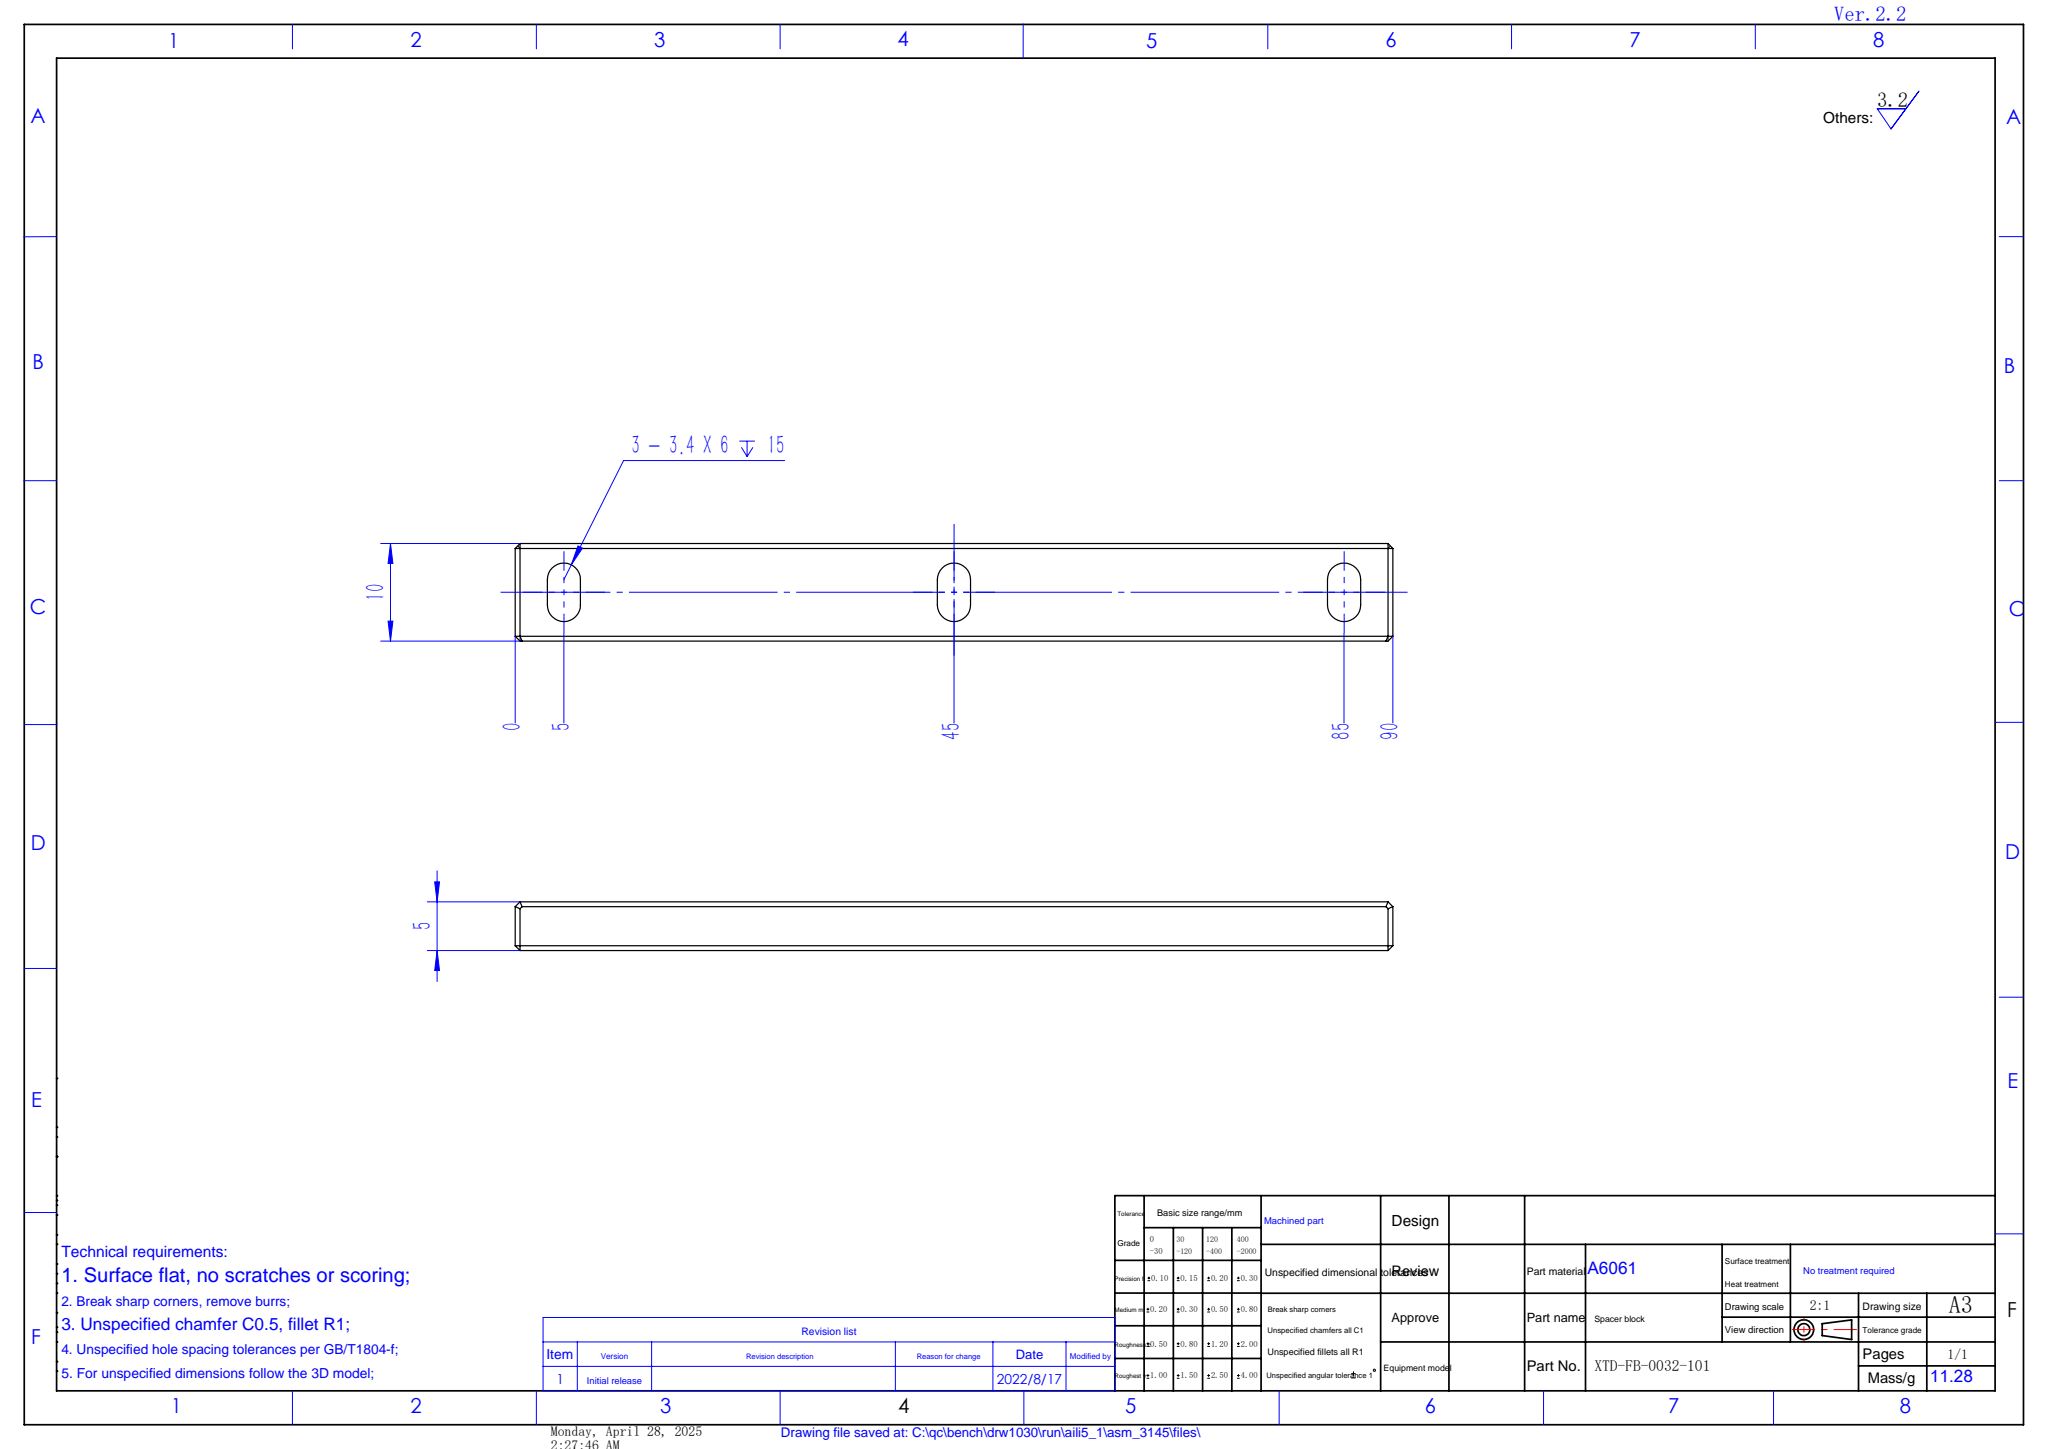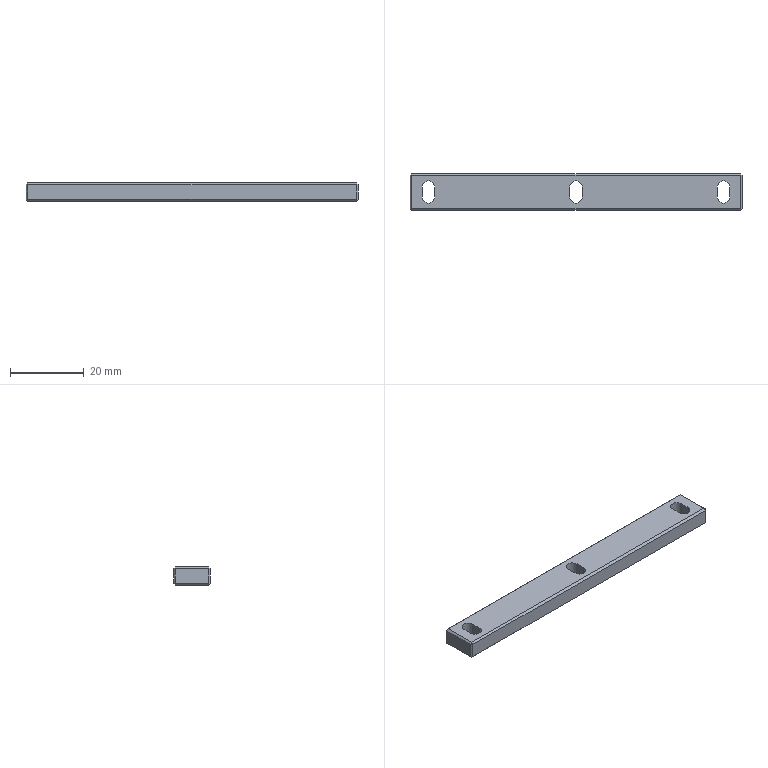Part | SolidWorks | features Chamfer 2, Extrusion 1, HoleWzd 1 | 1 solid | 36 faces | box 90 x 10 x 5 mm | volume 4179 mm3 | plane 30 | cylinder 6 | commonest cylinder face diameters 3.4 x6
STEP:
#1=CARTESIAN_POINT('',(44.5,-4.5,5.));
#2=VERTEX_POINT('',#1);
#3=CARTESIAN_POINT('',(44.5,4.5,5.));
#4=VERTEX_POINT('',#3);
#5=CARTESIAN_POINT('',(44.5,0.,5.));
#6=DIRECTION('',(0.,1.,0.));
#7=VECTOR('',#6,1000.);
#8=LINE('',#5,#7);
#9=EDGE_CURVE('',#2,#4,#8,.T.);
#10=ORIENTED_EDGE('',*,*,#9,.T.);
#11=CARTESIAN_POINT('',(-44.5,4.5,5.));
#12=VERTEX_POINT('',#11);
#13=CARTESIAN_POINT('',(0.,4.5,5.));
#14=DIRECTION('',(-1.,0.,0.));
#15=VECTOR('',#14,1000.);
#16=LINE('',#13,#15);
#17=EDGE_CURVE('',#4,#12,#16,.T.);
#18=ORIENTED_EDGE('',*,*,#17,.T.);
#19=CARTESIAN_POINT('',(-44.5,-4.5,5.));
#20=VERTEX_POINT('',#19);
#21=CARTESIAN_POINT('',(-44.5,0.,5.));
#22=DIRECTION('',(0.,-1.,0.));
#23=VECTOR('',#22,1000.);
#24=LINE('',#21,#23);
#25=EDGE_CURVE('',#12,#20,#24,.T.);
#26=ORIENTED_EDGE('',*,*,#25,.T.);
#27=CARTESIAN_POINT('',(0.,-4.5,5.));
#28=DIRECTION('',(1.,0.,0.));
#29=VECTOR('',#28,1000.);
#30=LINE('',#27,#29);
#31=EDGE_CURVE('',#20,#2,#30,.T.);
#32=ORIENTED_EDGE('',*,*,#31,.T.);
#33=EDGE_LOOP('',(#10,#18,#26,#32));
#34=FACE_OUTER_BOUND('',#33,.T.);
#35=CARTESIAN_POINT('',(1.7,-1.3,5.));
#36=VERTEX_POINT('',#35);
#37=CARTESIAN_POINT('',(-1.7,-1.3,5.));
#38=VERTEX_POINT('',#37);
#39=CARTESIAN_POINT('',(0.,-1.3,5.));
#40=DIRECTION('',(0.,0.,-1.));
#41=DIRECTION('',(-1.,0.,0.));
#42=AXIS2_PLACEMENT_3D('',#39,#40,#41);
#43=CIRCLE('',#42,1.7);
#44=EDGE_CURVE('',#36,#38,#43,.T.);
#45=ORIENTED_EDGE('',*,*,#44,.T.);
#46=CARTESIAN_POINT('',(-1.7,1.3,5.));
#47=VERTEX_POINT('',#46);
#48=CARTESIAN_POINT('',(-1.7,0.,5.));
#49=DIRECTION('',(0.,1.,0.));
#50=VECTOR('',#49,1000.);
#51=LINE('',#48,#50);
#52=EDGE_CURVE('',#38,#47,#51,.T.);
#53=ORIENTED_EDGE('',*,*,#52,.T.);
#54=CARTESIAN_POINT('',(1.7,1.3,5.));
#55=VERTEX_POINT('',#54);
#56=CARTESIAN_POINT('',(0.,1.3,5.));
#57=DIRECTION('',(0.,0.,-1.));
#58=DIRECTION('',(-1.,0.,0.));
#59=AXIS2_PLACEMENT_3D('',#56,#57,#58);
#60=CIRCLE('',#59,1.7);
#61=EDGE_CURVE('',#47,#55,#60,.T.);
#62=ORIENTED_EDGE('',*,*,#61,.T.);
#63=CARTESIAN_POINT('',(1.7,0.,5.));
#64=DIRECTION('',(0.,1.,0.));
#65=VECTOR('',#64,1000.);
#66=LINE('',#63,#65);
#67=EDGE_CURVE('',#36,#55,#66,.T.);
#68=ORIENTED_EDGE('',*,*,#67,.F.);
#69=EDGE_LOOP('',(#45,#53,#62,#68));
#70=FACE_BOUND('',#69,.T.);
#71=CARTESIAN_POINT('',(-41.7,-1.3,5.));
#72=VERTEX_POINT('',#71);
#73=CARTESIAN_POINT('',(-41.7,1.3,5.));
#74=VERTEX_POINT('',#73);
#75=CARTESIAN_POINT('',(-41.7,0.,5.));
#76=DIRECTION('',(0.,1.,0.));
#77=VECTOR('',#76,1000.);
#78=LINE('',#75,#77);
#79=EDGE_CURVE('',#72,#74,#78,.T.);
#80=ORIENTED_EDGE('',*,*,#79,.T.);
#81=CARTESIAN_POINT('',(-38.3,1.3,5.));
#82=VERTEX_POINT('',#81);
#83=CARTESIAN_POINT('',(-40.,1.3,5.));
#84=DIRECTION('',(0.,0.,-1.));
#85=DIRECTION('',(-1.,0.,0.));
#86=AXIS2_PLACEMENT_3D('',#83,#84,#85);
#87=CIRCLE('',#86,1.7);
#88=EDGE_CURVE('',#74,#82,#87,.T.);
#89=ORIENTED_EDGE('',*,*,#88,.T.);
#90=CARTESIAN_POINT('',(-38.3,-1.3,5.));
#91=VERTEX_POINT('',#90);
#92=CARTESIAN_POINT('',(-38.3,0.,5.));
#93=DIRECTION('',(0.,1.,0.));
#94=VECTOR('',#93,1000.);
#95=LINE('',#92,#94);
#96=EDGE_CURVE('',#91,#82,#95,.T.);
#97=ORIENTED_EDGE('',*,*,#96,.F.);
#98=CARTESIAN_POINT('',(-40.,-1.3,5.));
#99=DIRECTION('',(0.,0.,-1.));
#100=DIRECTION('',(-1.,0.,0.));
#101=AXIS2_PLACEMENT_3D('',#98,#99,#100);
#102=CIRCLE('',#101,1.7);
#103=EDGE_CURVE('',#91,#72,#102,.T.);
#104=ORIENTED_EDGE('',*,*,#103,.T.);
#105=EDGE_LOOP('',(#80,#89,#97,#104));
#106=FACE_BOUND('',#105,.T.);
#107=CARTESIAN_POINT('',(41.7,-1.3,5.));
#108=VERTEX_POINT('',#107);
#109=CARTESIAN_POINT('',(41.7,1.3,5.));
#110=VERTEX_POINT('',#109);
#111=CARTESIAN_POINT('',(41.7,0.,5.));
#112=DIRECTION('',(0.,1.,0.));
#113=VECTOR('',#112,1000.);
#114=LINE('',#111,#113);
#115=EDGE_CURVE('',#108,#110,#114,.T.);
#116=ORIENTED_EDGE('',*,*,#115,.F.);
#117=CARTESIAN_POINT('',(38.3,-1.3,5.));
#118=VERTEX_POINT('',#117);
#119=CARTESIAN_POINT('',(40.,-1.3,5.));
#120=DIRECTION('',(0.,0.,-1.));
#121=DIRECTION('',(-1.,0.,0.));
#122=AXIS2_PLACEMENT_3D('',#119,#120,#121);
#123=CIRCLE('',#122,1.7);
#124=EDGE_CURVE('',#108,#118,#123,.T.);
#125=ORIENTED_EDGE('',*,*,#124,.T.);
#126=CARTESIAN_POINT('',(38.3,1.3,5.));
#127=VERTEX_POINT('',#126);
#128=CARTESIAN_POINT('',(38.3,0.,5.));
#129=DIRECTION('',(0.,1.,0.));
#130=VECTOR('',#129,1000.);
#131=LINE('',#128,#130);
#132=EDGE_CURVE('',#118,#127,#131,.T.);
#133=ORIENTED_EDGE('',*,*,#132,.T.);
#134=CARTESIAN_POINT('',(40.,1.3,5.));
#135=DIRECTION('',(0.,0.,-1.));
#136=DIRECTION('',(-1.,0.,0.));
#137=AXIS2_PLACEMENT_3D('',#134,#135,#136);
#138=CIRCLE('',#137,1.7);
#139=EDGE_CURVE('',#127,#110,#138,.T.);
#140=ORIENTED_EDGE('',*,*,#139,.T.);
#141=EDGE_LOOP('',(#116,#125,#133,#140));
#142=FACE_BOUND('',#141,.T.);
#143=CARTESIAN_POINT('',(0.,0.,5.));
#144=DIRECTION('',(0.,0.,-1.));
#145=DIRECTION('',(-1.,0.,0.));
#146=AXIS2_PLACEMENT_3D('',#143,#144,#145);
#147=PLANE('',#146);
#148=ADVANCED_FACE('',(#34,#70,#106,#142),#147,.F.);
#149=CARTESIAN_POINT('',(45.,-4.5,4.5));
#150=VERTEX_POINT('',#149);
#151=CARTESIAN_POINT('',(45.,-4.5,0.5));
#152=VERTEX_POINT('',#151);
#153=CARTESIAN_POINT('',(45.,-4.5,5.));
#154=DIRECTION('',(0.,0.,-1.));
#155=VECTOR('',#154,1000.);
#156=LINE('',#153,#155);
#157=EDGE_CURVE('',#150,#152,#156,.T.);
#158=ORIENTED_EDGE('',*,*,#157,.T.);
#159=CARTESIAN_POINT('',(45.,4.5,0.5));
#160=VERTEX_POINT('',#159);
#161=CARTESIAN_POINT('',(45.,5.,0.5));
#162=DIRECTION('',(0.,1.,0.));
#163=VECTOR('',#162,1000.);
#164=LINE('',#161,#163);
#165=EDGE_CURVE('',#152,#160,#164,.T.);
#166=ORIENTED_EDGE('',*,*,#165,.T.);
#167=CARTESIAN_POINT('',(45.,4.5,4.5));
#168=VERTEX_POINT('',#167);
#169=CARTESIAN_POINT('',(45.,4.5,5.));
#170=DIRECTION('',(0.,0.,1.));
#171=VECTOR('',#170,1000.);
#172=LINE('',#169,#171);
#173=EDGE_CURVE('',#160,#168,#172,.T.);
#174=ORIENTED_EDGE('',*,*,#173,.T.);
#175=CARTESIAN_POINT('',(45.,-5.,4.5));
#176=DIRECTION('',(0.,-1.,0.));
#177=VECTOR('',#176,1000.);
#178=LINE('',#175,#177);
#179=EDGE_CURVE('',#168,#150,#178,.T.);
#180=ORIENTED_EDGE('',*,*,#179,.T.);
#181=EDGE_LOOP('',(#158,#166,#174,#180));
#182=FACE_OUTER_BOUND('',#181,.T.);
#183=CARTESIAN_POINT('',(45.,-5.,5.));
#184=DIRECTION('',(-1.,0.,0.));
#185=DIRECTION('',(0.,0.,1.));
#186=AXIS2_PLACEMENT_3D('',#183,#184,#185);
#187=PLANE('',#186);
#188=ADVANCED_FACE('',(#182),#187,.F.);
#189=CARTESIAN_POINT('',(44.5,5.,4.293));
#190=VERTEX_POINT('',#189);
#191=CARTESIAN_POINT('',(44.5,5.,0.5));
#192=VERTEX_POINT('',#191);
#193=CARTESIAN_POINT('',(44.5,5.,5.));
#194=DIRECTION('',(0.,0.,-1.));
#195=VECTOR('',#194,1000.);
#196=LINE('',#193,#195);
#197=EDGE_CURVE('',#190,#192,#196,.T.);
#198=ORIENTED_EDGE('',*,*,#197,.T.);
#199=CARTESIAN_POINT('',(-44.5,5.,0.5));
#200=VERTEX_POINT('',#199);
#201=CARTESIAN_POINT('',(-45.,5.,0.5));
#202=DIRECTION('',(-1.,0.,0.));
#203=VECTOR('',#202,1000.);
#204=LINE('',#201,#203);
#205=EDGE_CURVE('',#192,#200,#204,.T.);
#206=ORIENTED_EDGE('',*,*,#205,.T.);
#207=CARTESIAN_POINT('',(-44.5,5.,4.293));
#208=VERTEX_POINT('',#207);
#209=CARTESIAN_POINT('',(-44.5,5.,5.));
#210=DIRECTION('',(0.,0.,1.));
#211=VECTOR('',#210,1000.);
#212=LINE('',#209,#211);
#213=EDGE_CURVE('',#200,#208,#212,.T.);
#214=ORIENTED_EDGE('',*,*,#213,.T.);
#215=CARTESIAN_POINT('',(-44.293,5.,4.5));
#216=VERTEX_POINT('',#215);
#217=CARTESIAN_POINT('',(-44.146,5.,4.646));
#218=DIRECTION('',(0.7071,0.,0.7071));
#219=VECTOR('',#218,1000.);
#220=LINE('',#217,#219);
#221=EDGE_CURVE('',#208,#216,#220,.T.);
#222=ORIENTED_EDGE('',*,*,#221,.T.);
#223=CARTESIAN_POINT('',(44.293,5.,4.5));
#224=VERTEX_POINT('',#223);
#225=CARTESIAN_POINT('',(-45.,5.,4.5));
#226=DIRECTION('',(1.,0.,0.));
#227=VECTOR('',#226,1000.);
#228=LINE('',#225,#227);
#229=EDGE_CURVE('',#216,#224,#228,.T.);
#230=ORIENTED_EDGE('',*,*,#229,.T.);
#231=CARTESIAN_POINT('',(44.646,5.,4.146));
#232=DIRECTION('',(0.7071,0.,-0.7071));
#233=VECTOR('',#232,1000.);
#234=LINE('',#231,#233);
#235=EDGE_CURVE('',#224,#190,#234,.T.);
#236=ORIENTED_EDGE('',*,*,#235,.T.);
#237=EDGE_LOOP('',(#198,#206,#214,#222,#230,#236));
#238=FACE_OUTER_BOUND('',#237,.T.);
#239=CARTESIAN_POINT('',(-45.,5.,5.));
#240=DIRECTION('',(0.,-1.,0.));
#241=DIRECTION('',(0.,0.,-1.));
#242=AXIS2_PLACEMENT_3D('',#239,#240,#241);
#243=PLANE('',#242);
#244=ADVANCED_FACE('',(#238),#243,.F.);
#245=CARTESIAN_POINT('',(-45.,-4.5,4.5));
#246=VERTEX_POINT('',#245);
#247=CARTESIAN_POINT('',(-45.,4.5,4.5));
#248=VERTEX_POINT('',#247);
#249=CARTESIAN_POINT('',(-45.,-5.,4.5));
#250=DIRECTION('',(0.,1.,0.));
#251=VECTOR('',#250,1000.);
#252=LINE('',#249,#251);
#253=EDGE_CURVE('',#246,#248,#252,.T.);
#254=ORIENTED_EDGE('',*,*,#253,.T.);
#255=CARTESIAN_POINT('',(-45.,4.5,0.5));
#256=VERTEX_POINT('',#255);
#257=CARTESIAN_POINT('',(-45.,4.5,5.));
#258=DIRECTION('',(0.,0.,-1.));
#259=VECTOR('',#258,1000.);
#260=LINE('',#257,#259);
#261=EDGE_CURVE('',#248,#256,#260,.T.);
#262=ORIENTED_EDGE('',*,*,#261,.T.);
#263=CARTESIAN_POINT('',(-45.,-4.5,0.5));
#264=VERTEX_POINT('',#263);
#265=CARTESIAN_POINT('',(-45.,-4.5,0.5));
#266=DIRECTION('',(0.,-1.,0.));
#267=VECTOR('',#266,1000.);
#268=LINE('',#265,#267);
#269=EDGE_CURVE('',#256,#264,#268,.T.);
#270=ORIENTED_EDGE('',*,*,#269,.T.);
#271=CARTESIAN_POINT('',(-45.,-4.5,5.));
#272=DIRECTION('',(0.,0.,1.));
#273=VECTOR('',#272,1000.);
#274=LINE('',#271,#273);
#275=EDGE_CURVE('',#264,#246,#274,.T.);
#276=ORIENTED_EDGE('',*,*,#275,.T.);
#277=EDGE_LOOP('',(#254,#262,#270,#276));
#278=FACE_OUTER_BOUND('',#277,.T.);
#279=CARTESIAN_POINT('',(-45.,-5.,5.));
#280=DIRECTION('',(1.,0.,0.));
#281=DIRECTION('',(0.,0.,-1.));
#282=AXIS2_PLACEMENT_3D('',#279,#280,#281);
#283=PLANE('',#282);
#284=ADVANCED_FACE('',(#278),#283,.F.);
#285=CARTESIAN_POINT('',(44.5,-5.,4.5));
#286=VERTEX_POINT('',#285);
#287=CARTESIAN_POINT('',(-44.5,-5.,4.5));
#288=VERTEX_POINT('',#287);
#289=CARTESIAN_POINT('',(-45.,-5.,4.5));
#290=DIRECTION('',(-1.,0.,0.));
#291=VECTOR('',#290,1000.);
#292=LINE('',#289,#291);
#293=EDGE_CURVE('',#286,#288,#292,.T.);
#294=ORIENTED_EDGE('',*,*,#293,.T.);
#295=CARTESIAN_POINT('',(-44.5,-5.,0.5));
#296=VERTEX_POINT('',#295);
#297=CARTESIAN_POINT('',(-44.5,-5.,5.));
#298=DIRECTION('',(0.,0.,-1.));
#299=VECTOR('',#298,1000.);
#300=LINE('',#297,#299);
#301=EDGE_CURVE('',#288,#296,#300,.T.);
#302=ORIENTED_EDGE('',*,*,#301,.T.);
#303=CARTESIAN_POINT('',(44.5,-5.,0.5));
#304=VERTEX_POINT('',#303);
#305=CARTESIAN_POINT('',(45.,-5.,0.5));
#306=DIRECTION('',(1.,0.,0.));
#307=VECTOR('',#306,1000.);
#308=LINE('',#305,#307);
#309=EDGE_CURVE('',#296,#304,#308,.T.);
#310=ORIENTED_EDGE('',*,*,#309,.T.);
#311=CARTESIAN_POINT('',(44.5,-5.,5.));
#312=DIRECTION('',(0.,0.,1.));
#313=VECTOR('',#312,1000.);
#314=LINE('',#311,#313);
#315=EDGE_CURVE('',#304,#286,#314,.T.);
#316=ORIENTED_EDGE('',*,*,#315,.T.);
#317=EDGE_LOOP('',(#294,#302,#310,#316));
#318=FACE_OUTER_BOUND('',#317,.T.);
#319=CARTESIAN_POINT('',(-45.,-5.,5.));
#320=DIRECTION('',(0.,1.,0.));
#321=DIRECTION('',(0.,0.,1.));
#322=AXIS2_PLACEMENT_3D('',#319,#320,#321);
#323=PLANE('',#322);
#324=ADVANCED_FACE('',(#318),#323,.F.);
#325=CARTESIAN_POINT('',(38.3,-1.3,0.));
#326=VERTEX_POINT('',#325);
#327=CARTESIAN_POINT('',(38.3,1.3,0.));
#328=VERTEX_POINT('',#327);
#329=CARTESIAN_POINT('',(38.3,-1.3,0.));
#330=DIRECTION('',(0.,1.,0.));
#331=VECTOR('',#330,1000.);
#332=LINE('',#329,#331);
#333=EDGE_CURVE('',#326,#328,#332,.T.);
#334=ORIENTED_EDGE('',*,*,#333,.F.);
#335=CARTESIAN_POINT('',(41.7,-1.3,0.));
#336=VERTEX_POINT('',#335);
#337=CARTESIAN_POINT('',(40.,-1.3,0.));
#338=DIRECTION('',(0.,0.,-1.));
#339=DIRECTION('',(-1.,0.,0.));
#340=AXIS2_PLACEMENT_3D('',#337,#338,#339);
#341=CIRCLE('',#340,1.7);
#342=EDGE_CURVE('',#336,#326,#341,.T.);
#343=ORIENTED_EDGE('',*,*,#342,.F.);
#344=CARTESIAN_POINT('',(41.7,1.3,0.));
#345=VERTEX_POINT('',#344);
#346=CARTESIAN_POINT('',(41.7,-1.3,0.));
#347=DIRECTION('',(0.,1.,0.));
#348=VECTOR('',#347,1000.);
#349=LINE('',#346,#348);
#350=EDGE_CURVE('',#336,#345,#349,.T.);
#351=ORIENTED_EDGE('',*,*,#350,.T.);
#352=CARTESIAN_POINT('',(40.,1.3,0.));
#353=DIRECTION('',(0.,0.,-1.));
#354=DIRECTION('',(-1.,0.,0.));
#355=AXIS2_PLACEMENT_3D('',#352,#353,#354);
#356=CIRCLE('',#355,1.7);
#357=EDGE_CURVE('',#328,#345,#356,.T.);
#358=ORIENTED_EDGE('',*,*,#357,.F.);
#359=EDGE_LOOP('',(#334,#343,#351,#358));
#360=FACE_BOUND('',#359,.T.);
#361=CARTESIAN_POINT('',(-41.7,1.3,0.));
#362=VERTEX_POINT('',#361);
#363=CARTESIAN_POINT('',(-38.3,1.3,0.));
#364=VERTEX_POINT('',#363);
#365=CARTESIAN_POINT('',(-40.,1.3,0.));
#366=DIRECTION('',(0.,0.,-1.));
#367=DIRECTION('',(-1.,0.,0.));
#368=AXIS2_PLACEMENT_3D('',#365,#366,#367);
#369=CIRCLE('',#368,1.7);
#370=EDGE_CURVE('',#362,#364,#369,.T.);
#371=ORIENTED_EDGE('',*,*,#370,.F.);
#372=CARTESIAN_POINT('',(-41.7,-1.3,0.));
#373=VERTEX_POINT('',#372);
#374=CARTESIAN_POINT('',(-41.7,-1.3,0.));
#375=DIRECTION('',(0.,1.,0.));
#376=VECTOR('',#375,1000.);
#377=LINE('',#374,#376);
#378=EDGE_CURVE('',#373,#362,#377,.T.);
#379=ORIENTED_EDGE('',*,*,#378,.F.);
#380=CARTESIAN_POINT('',(-38.3,-1.3,0.));
#381=VERTEX_POINT('',#380);
#382=CARTESIAN_POINT('',(-40.,-1.3,0.));
#383=DIRECTION('',(0.,0.,-1.));
#384=DIRECTION('',(-1.,0.,0.));
#385=AXIS2_PLACEMENT_3D('',#382,#383,#384);
#386=CIRCLE('',#385,1.7);
#387=EDGE_CURVE('',#381,#373,#386,.T.);
#388=ORIENTED_EDGE('',*,*,#387,.F.);
#389=CARTESIAN_POINT('',(-38.3,-1.3,0.));
#390=DIRECTION('',(0.,1.,0.));
#391=VECTOR('',#390,1000.);
#392=LINE('',#389,#391);
#393=EDGE_CURVE('',#381,#364,#392,.T.);
#394=ORIENTED_EDGE('',*,*,#393,.T.);
#395=EDGE_LOOP('',(#371,#379,#388,#394));
#396=FACE_BOUND('',#395,.T.);
#397=CARTESIAN_POINT('',(1.7,-1.3,0.));
#398=VERTEX_POINT('',#397);
#399=CARTESIAN_POINT('',(-1.7,-1.3,0.));
#400=VERTEX_POINT('',#399);
#401=CARTESIAN_POINT('',(0.,-1.3,0.));
#402=DIRECTION('',(0.,0.,-1.));
#403=DIRECTION('',(-1.,0.,0.));
#404=AXIS2_PLACEMENT_3D('',#401,#402,#403);
#405=CIRCLE('',#404,1.7);
#406=EDGE_CURVE('',#398,#400,#405,.T.);
#407=ORIENTED_EDGE('',*,*,#406,.F.);
#408=CARTESIAN_POINT('',(1.7,1.3,0.));
#409=VERTEX_POINT('',#408);
#410=CARTESIAN_POINT('',(1.7,-1.3,0.));
#411=DIRECTION('',(0.,1.,0.));
#412=VECTOR('',#411,1000.);
#413=LINE('',#410,#412);
#414=EDGE_CURVE('',#398,#409,#413,.T.);
#415=ORIENTED_EDGE('',*,*,#414,.T.);
#416=CARTESIAN_POINT('',(-1.7,1.3,0.));
#417=VERTEX_POINT('',#416);
#418=CARTESIAN_POINT('',(0.,1.3,0.));
#419=DIRECTION('',(0.,0.,-1.));
#420=DIRECTION('',(-1.,0.,0.));
#421=AXIS2_PLACEMENT_3D('',#418,#419,#420);
#422=CIRCLE('',#421,1.7);
#423=EDGE_CURVE('',#417,#409,#422,.T.);
#424=ORIENTED_EDGE('',*,*,#423,.F.);
#425=CARTESIAN_POINT('',(-1.7,-1.3,0.));
#426=DIRECTION('',(0.,1.,0.));
#427=VECTOR('',#426,1000.);
#428=LINE('',#425,#427);
#429=EDGE_CURVE('',#400,#417,#428,.T.);
#430=ORIENTED_EDGE('',*,*,#429,.F.);
#431=EDGE_LOOP('',(#407,#415,#424,#430));
#432=FACE_BOUND('',#431,.T.);
#433=CARTESIAN_POINT('',(-44.5,4.5,0.));
#434=VERTEX_POINT('',#433);
#435=CARTESIAN_POINT('',(44.5,4.5,0.));
#436=VERTEX_POINT('',#435);
#437=CARTESIAN_POINT('',(45.,4.5,0.));
#438=DIRECTION('',(1.,0.,0.));
#439=VECTOR('',#438,1000.);
#440=LINE('',#437,#439);
#441=EDGE_CURVE('',#434,#436,#440,.T.);
#442=ORIENTED_EDGE('',*,*,#441,.T.);
#443=CARTESIAN_POINT('',(44.5,-4.5,0.));
#444=VERTEX_POINT('',#443);
#445=CARTESIAN_POINT('',(44.5,-4.5,0.));
#446=DIRECTION('',(0.,-1.,0.));
#447=VECTOR('',#446,1000.);
#448=LINE('',#445,#447);
#449=EDGE_CURVE('',#436,#444,#448,.T.);
#450=ORIENTED_EDGE('',*,*,#449,.T.);
#451=CARTESIAN_POINT('',(-44.5,-4.5,0.));
#452=VERTEX_POINT('',#451);
#453=CARTESIAN_POINT('',(-45.,-4.5,0.));
#454=DIRECTION('',(-1.,0.,0.));
#455=VECTOR('',#454,1000.);
#456=LINE('',#453,#455);
#457=EDGE_CURVE('',#444,#452,#456,.T.);
#458=ORIENTED_EDGE('',*,*,#457,.T.);
#459=CARTESIAN_POINT('',(-44.5,5.,0.));
#460=DIRECTION('',(0.,1.,0.));
#461=VECTOR('',#460,1000.);
#462=LINE('',#459,#461);
#463=EDGE_CURVE('',#452,#434,#462,.T.);
#464=ORIENTED_EDGE('',*,*,#463,.T.);
#465=EDGE_LOOP('',(#442,#450,#458,#464));
#466=FACE_OUTER_BOUND('',#465,.T.);
#467=CARTESIAN_POINT('',(0.,0.,0.));
#468=DIRECTION('',(0.,0.,-1.));
#469=DIRECTION('',(-1.,0.,0.));
#470=AXIS2_PLACEMENT_3D('',#467,#468,#469);
#471=PLANE('',#470);
#472=ADVANCED_FACE('',(#360,#396,#432,#466),#471,.T.);
#473=CARTESIAN_POINT('',(1.7,-1.3,15.));
#474=DIRECTION('',(0.,0.,1.));
#475=VECTOR('',#474,1000.);
#476=LINE('',#473,#475);
#477=EDGE_CURVE('',#398,#36,#476,.T.);
#478=ORIENTED_EDGE('',*,*,#477,.F.);
#479=ORIENTED_EDGE('',*,*,#406,.T.);
#480=CARTESIAN_POINT('',(-1.7,-1.3,0.));
#481=DIRECTION('',(0.,0.,-1.));
#482=VECTOR('',#481,1000.);
#483=LINE('',#480,#482);
#484=EDGE_CURVE('',#38,#400,#483,.T.);
#485=ORIENTED_EDGE('',*,*,#484,.F.);
#486=ORIENTED_EDGE('',*,*,#44,.F.);
#487=EDGE_LOOP('',(#478,#479,#485,#486));
#488=FACE_OUTER_BOUND('',#487,.T.);
#489=CARTESIAN_POINT('',(0.,-1.3,0.));
#490=DIRECTION('',(0.,0.,-1.));
#491=DIRECTION('',(-1.,0.,0.));
#492=AXIS2_PLACEMENT_3D('',#489,#490,#491);
#493=CYLINDRICAL_SURFACE('',#492,1.7);
#494=ADVANCED_FACE('',(#488),#493,.F.);
#495=ORIENTED_EDGE('',*,*,#67,.T.);
#496=CARTESIAN_POINT('',(1.7,1.3,15.));
#497=DIRECTION('',(0.,0.,1.));
#498=VECTOR('',#497,1000.);
#499=LINE('',#496,#498);
#500=EDGE_CURVE('',#409,#55,#499,.T.);
#501=ORIENTED_EDGE('',*,*,#500,.F.);
#502=ORIENTED_EDGE('',*,*,#414,.F.);
#503=ORIENTED_EDGE('',*,*,#477,.T.);
#504=EDGE_LOOP('',(#495,#501,#502,#503));
#505=FACE_OUTER_BOUND('',#504,.T.);
#506=CARTESIAN_POINT('',(1.7,-1.3,15.));
#507=DIRECTION('',(-1.,0.,0.));
#508=DIRECTION('',(0.,0.,1.));
#509=AXIS2_PLACEMENT_3D('',#506,#507,#508);
#510=PLANE('',#509);
#511=ADVANCED_FACE('',(#505),#510,.T.);
#512=CARTESIAN_POINT('',(-1.7,1.3,0.));
#513=DIRECTION('',(0.,0.,1.));
#514=VECTOR('',#513,1000.);
#515=LINE('',#512,#514);
#516=EDGE_CURVE('',#417,#47,#515,.T.);
#517=ORIENTED_EDGE('',*,*,#516,.F.);
#518=ORIENTED_EDGE('',*,*,#423,.T.);
#519=ORIENTED_EDGE('',*,*,#500,.T.);
#520=ORIENTED_EDGE('',*,*,#61,.F.);
#521=EDGE_LOOP('',(#517,#518,#519,#520));
#522=FACE_OUTER_BOUND('',#521,.T.);
#523=CARTESIAN_POINT('',(0.,1.3,0.));
#524=DIRECTION('',(0.,0.,-1.));
#525=DIRECTION('',(-1.,0.,0.));
#526=AXIS2_PLACEMENT_3D('',#523,#524,#525);
#527=CYLINDRICAL_SURFACE('',#526,1.7);
#528=ADVANCED_FACE('',(#522),#527,.F.);
#529=ORIENTED_EDGE('',*,*,#484,.T.);
#530=ORIENTED_EDGE('',*,*,#429,.T.);
#531=ORIENTED_EDGE('',*,*,#516,.T.);
#532=ORIENTED_EDGE('',*,*,#52,.F.);
#533=EDGE_LOOP('',(#529,#530,#531,#532));
#534=FACE_OUTER_BOUND('',#533,.T.);
#535=CARTESIAN_POINT('',(-1.7,-1.3,0.));
#536=DIRECTION('',(-1.,0.,0.));
#537=DIRECTION('',(0.,0.,1.));
#538=AXIS2_PLACEMENT_3D('',#535,#536,#537);
#539=PLANE('',#538);
#540=ADVANCED_FACE('',(#534),#539,.F.);
#541=CARTESIAN_POINT('',(-38.3,-1.3,15.));
#542=DIRECTION('',(0.,0.,1.));
#543=VECTOR('',#542,1000.);
#544=LINE('',#541,#543);
#545=EDGE_CURVE('',#381,#91,#544,.T.);
#546=ORIENTED_EDGE('',*,*,#545,.F.);
#547=ORIENTED_EDGE('',*,*,#387,.T.);
#548=CARTESIAN_POINT('',(-41.7,-1.3,0.));
#549=DIRECTION('',(0.,0.,-1.));
#550=VECTOR('',#549,1000.);
#551=LINE('',#548,#550);
#552=EDGE_CURVE('',#72,#373,#551,.T.);
#553=ORIENTED_EDGE('',*,*,#552,.F.);
#554=ORIENTED_EDGE('',*,*,#103,.F.);
#555=EDGE_LOOP('',(#546,#547,#553,#554));
#556=FACE_OUTER_BOUND('',#555,.T.);
#557=CARTESIAN_POINT('',(-40.,-1.3,0.));
#558=DIRECTION('',(0.,0.,-1.));
#559=DIRECTION('',(-1.,0.,0.));
#560=AXIS2_PLACEMENT_3D('',#557,#558,#559);
#561=CYLINDRICAL_SURFACE('',#560,1.7);
#562=ADVANCED_FACE('',(#556),#561,.F.);
#563=CARTESIAN_POINT('',(-41.7,1.3,0.));
#564=DIRECTION('',(0.,0.,1.));
#565=VECTOR('',#564,1000.);
#566=LINE('',#563,#565);
#567=EDGE_CURVE('',#362,#74,#566,.T.);
#568=ORIENTED_EDGE('',*,*,#567,.F.);
#569=ORIENTED_EDGE('',*,*,#370,.T.);
#570=CARTESIAN_POINT('',(-38.3,1.3,15.));
#571=DIRECTION('',(0.,0.,1.));
#572=VECTOR('',#571,1000.);
#573=LINE('',#570,#572);
#574=EDGE_CURVE('',#364,#82,#573,.T.);
#575=ORIENTED_EDGE('',*,*,#574,.T.);
#576=ORIENTED_EDGE('',*,*,#88,.F.);
#577=EDGE_LOOP('',(#568,#569,#575,#576));
#578=FACE_OUTER_BOUND('',#577,.T.);
#579=CARTESIAN_POINT('',(-40.,1.3,0.));
#580=DIRECTION('',(0.,0.,-1.));
#581=DIRECTION('',(-1.,0.,0.));
#582=AXIS2_PLACEMENT_3D('',#579,#580,#581);
#583=CYLINDRICAL_SURFACE('',#582,1.7);
#584=ADVANCED_FACE('',(#578),#583,.F.);
#585=ORIENTED_EDGE('',*,*,#552,.T.);
#586=ORIENTED_EDGE('',*,*,#378,.T.);
#587=ORIENTED_EDGE('',*,*,#567,.T.);
#588=ORIENTED_EDGE('',*,*,#79,.F.);
#589=EDGE_LOOP('',(#585,#586,#587,#588));
#590=FACE_OUTER_BOUND('',#589,.T.);
#591=CARTESIAN_POINT('',(-41.7,-1.3,0.));
#592=DIRECTION('',(-1.,0.,0.));
#593=DIRECTION('',(0.,0.,1.));
#594=AXIS2_PLACEMENT_3D('',#591,#592,#593);
#595=PLANE('',#594);
#596=ADVANCED_FACE('',(#590),#595,.F.);
#597=ORIENTED_EDGE('',*,*,#96,.T.);
#598=ORIENTED_EDGE('',*,*,#574,.F.);
#599=ORIENTED_EDGE('',*,*,#393,.F.);
#600=ORIENTED_EDGE('',*,*,#545,.T.);
#601=EDGE_LOOP('',(#597,#598,#599,#600));
#602=FACE_OUTER_BOUND('',#601,.T.);
#603=CARTESIAN_POINT('',(-38.3,-1.3,15.));
#604=DIRECTION('',(-1.,0.,0.));
#605=DIRECTION('',(0.,0.,1.));
#606=AXIS2_PLACEMENT_3D('',#603,#604,#605);
#607=PLANE('',#606);
#608=ADVANCED_FACE('',(#602),#607,.T.);
#609=CARTESIAN_POINT('',(38.3,1.3,0.));
#610=DIRECTION('',(0.,0.,1.));
#611=VECTOR('',#610,1000.);
#612=LINE('',#609,#611);
#613=EDGE_CURVE('',#328,#127,#612,.T.);
#614=ORIENTED_EDGE('',*,*,#613,.F.);
#615=ORIENTED_EDGE('',*,*,#357,.T.);
#616=CARTESIAN_POINT('',(41.7,1.3,15.));
#617=DIRECTION('',(0.,0.,1.));
#618=VECTOR('',#617,1000.);
#619=LINE('',#616,#618);
#620=EDGE_CURVE('',#345,#110,#619,.T.);
#621=ORIENTED_EDGE('',*,*,#620,.T.);
#622=ORIENTED_EDGE('',*,*,#139,.F.);
#623=EDGE_LOOP('',(#614,#615,#621,#622));
#624=FACE_OUTER_BOUND('',#623,.T.);
#625=CARTESIAN_POINT('',(40.,1.3,0.));
#626=DIRECTION('',(0.,0.,-1.));
#627=DIRECTION('',(-1.,0.,0.));
#628=AXIS2_PLACEMENT_3D('',#625,#626,#627);
#629=CYLINDRICAL_SURFACE('',#628,1.7);
#630=ADVANCED_FACE('',(#624),#629,.F.);
#631=ORIENTED_EDGE('',*,*,#115,.T.);
#632=ORIENTED_EDGE('',*,*,#620,.F.);
#633=ORIENTED_EDGE('',*,*,#350,.F.);
#634=CARTESIAN_POINT('',(41.7,-1.3,15.));
#635=DIRECTION('',(0.,0.,1.));
#636=VECTOR('',#635,1000.);
#637=LINE('',#634,#636);
#638=EDGE_CURVE('',#336,#108,#637,.T.);
#639=ORIENTED_EDGE('',*,*,#638,.T.);
#640=EDGE_LOOP('',(#631,#632,#633,#639));
#641=FACE_OUTER_BOUND('',#640,.T.);
#642=CARTESIAN_POINT('',(41.7,-1.3,15.));
#643=DIRECTION('',(-1.,0.,0.));
#644=DIRECTION('',(0.,0.,1.));
#645=AXIS2_PLACEMENT_3D('',#642,#643,#644);
#646=PLANE('',#645);
#647=ADVANCED_FACE('',(#641),#646,.T.);
#648=CARTESIAN_POINT('',(38.3,-1.3,0.));
#649=DIRECTION('',(0.,0.,-1.));
#650=VECTOR('',#649,1000.);
#651=LINE('',#648,#650);
#652=EDGE_CURVE('',#118,#326,#651,.T.);
#653=ORIENTED_EDGE('',*,*,#652,.T.);
#654=ORIENTED_EDGE('',*,*,#333,.T.);
#655=ORIENTED_EDGE('',*,*,#613,.T.);
#656=ORIENTED_EDGE('',*,*,#132,.F.);
#657=EDGE_LOOP('',(#653,#654,#655,#656));
#658=FACE_OUTER_BOUND('',#657,.T.);
#659=CARTESIAN_POINT('',(38.3,-1.3,0.));
#660=DIRECTION('',(-1.,0.,0.));
#661=DIRECTION('',(0.,0.,1.));
#662=AXIS2_PLACEMENT_3D('',#659,#660,#661);
#663=PLANE('',#662);
#664=ADVANCED_FACE('',(#658),#663,.F.);
#665=ORIENTED_EDGE('',*,*,#638,.F.);
#666=ORIENTED_EDGE('',*,*,#342,.T.);
#667=ORIENTED_EDGE('',*,*,#652,.F.);
#668=ORIENTED_EDGE('',*,*,#124,.F.);
#669=EDGE_LOOP('',(#665,#666,#667,#668));
#670=FACE_OUTER_BOUND('',#669,.T.);
#671=CARTESIAN_POINT('',(40.,-1.3,0.));
#672=DIRECTION('',(0.,0.,-1.));
#673=DIRECTION('',(-1.,0.,0.));
#674=AXIS2_PLACEMENT_3D('',#671,#672,#673);
#675=CYLINDRICAL_SURFACE('',#674,1.7);
#676=ADVANCED_FACE('',(#670),#675,.F.);
#677=ORIENTED_EDGE('',*,*,#179,.F.);
#678=CARTESIAN_POINT('',(44.5,4.5,5.));
#679=DIRECTION('',(-0.7071,0.,0.7071));
#680=VECTOR('',#679,1000.);
#681=LINE('',#678,#680);
#682=EDGE_CURVE('',#168,#4,#681,.T.);
#683=ORIENTED_EDGE('',*,*,#682,.T.);
#684=ORIENTED_EDGE('',*,*,#9,.F.);
#685=CARTESIAN_POINT('',(44.5,-4.5,5.));
#686=DIRECTION('',(-0.7071,0.,0.7071));
#687=VECTOR('',#686,1000.);
#688=LINE('',#685,#687);
#689=EDGE_CURVE('',#150,#2,#688,.T.);
#690=ORIENTED_EDGE('',*,*,#689,.F.);
#691=EDGE_LOOP('',(#677,#683,#684,#690));
#692=FACE_OUTER_BOUND('',#691,.T.);
#693=CARTESIAN_POINT('',(44.5,0.,5.));
#694=DIRECTION('',(-0.7071,0.,-0.7071));
#695=DIRECTION('',(0.,1.,0.));
#696=AXIS2_PLACEMENT_3D('',#693,#694,#695);
#697=PLANE('',#696);
#698=ADVANCED_FACE('',(#692),#697,.F.);
#699=CARTESIAN_POINT('',(44.75,-4.75,4.5));
#700=DIRECTION('',(-0.7071,-0.7071,0.));
#701=VECTOR('',#700,1000.);
#702=LINE('',#699,#701);
#703=EDGE_CURVE('',#150,#286,#702,.T.);
#704=ORIENTED_EDGE('',*,*,#703,.F.);
#705=ORIENTED_EDGE('',*,*,#689,.T.);
#706=CARTESIAN_POINT('',(44.5,-4.5,5.));
#707=DIRECTION('',(0.,0.7071,0.7071));
#708=VECTOR('',#707,1000.);
#709=LINE('',#706,#708);
#710=EDGE_CURVE('',#286,#2,#709,.T.);
#711=ORIENTED_EDGE('',*,*,#710,.F.);
#712=EDGE_LOOP('',(#704,#705,#711));
#713=FACE_OUTER_BOUND('',#712,.T.);
#714=CARTESIAN_POINT('',(44.5,-4.5,5.));
#715=DIRECTION('',(0.5774,-0.5774,0.5774));
#716=DIRECTION('',(0.7071,0.,-0.7071));
#717=AXIS2_PLACEMENT_3D('',#714,#715,#716);
#718=PLANE('',#717);
#719=ADVANCED_FACE('',(#713),#718,.T.);
#720=ORIENTED_EDGE('',*,*,#25,.F.);
#721=CARTESIAN_POINT('',(-45.,4.5,4.5));
#722=DIRECTION('',(-0.7071,0.,-0.7071));
#723=VECTOR('',#722,1000.);
#724=LINE('',#721,#723);
#725=EDGE_CURVE('',#12,#248,#724,.T.);
#726=ORIENTED_EDGE('',*,*,#725,.T.);
#727=ORIENTED_EDGE('',*,*,#253,.F.);
#728=CARTESIAN_POINT('',(-45.,-4.5,4.5));
#729=DIRECTION('',(-0.7071,0.,-0.7071));
#730=VECTOR('',#729,1000.);
#731=LINE('',#728,#730);
#732=EDGE_CURVE('',#20,#246,#731,.T.);
#733=ORIENTED_EDGE('',*,*,#732,.F.);
#734=EDGE_LOOP('',(#720,#726,#727,#733));
#735=FACE_OUTER_BOUND('',#734,.T.);
#736=CARTESIAN_POINT('',(-44.5,0.,5.));
#737=DIRECTION('',(0.7071,0.,-0.7071));
#738=DIRECTION('',(0.,-1.,0.));
#739=AXIS2_PLACEMENT_3D('',#736,#737,#738);
#740=PLANE('',#739);
#741=ADVANCED_FACE('',(#735),#740,.F.);
#742=ORIENTED_EDGE('',*,*,#710,.T.);
#743=ORIENTED_EDGE('',*,*,#31,.F.);
#744=CARTESIAN_POINT('',(-44.5,-4.75,4.75));
#745=DIRECTION('',(0.,0.7071,0.7071));
#746=VECTOR('',#745,1000.);
#747=LINE('',#744,#746);
#748=EDGE_CURVE('',#288,#20,#747,.T.);
#749=ORIENTED_EDGE('',*,*,#748,.F.);
#750=ORIENTED_EDGE('',*,*,#293,.F.);
#751=EDGE_LOOP('',(#742,#743,#749,#750));
#752=FACE_OUTER_BOUND('',#751,.T.);
#753=CARTESIAN_POINT('',(0.,-4.5,5.));
#754=DIRECTION('',(0.,0.7071,-0.7071));
#755=DIRECTION('',(1.,0.,0.));
#756=AXIS2_PLACEMENT_3D('',#753,#754,#755);
#757=PLANE('',#756);
#758=ADVANCED_FACE('',(#752),#757,.F.);
#759=CARTESIAN_POINT('',(44.75,-4.75,0.25));
#760=VERTEX_POINT('',#759);
#761=CARTESIAN_POINT('',(43.333,-6.167,1.667));
#762=DIRECTION('',(-0.5774,-0.5774,0.5774));
#763=VECTOR('',#762,1000.);
#764=LINE('',#761,#763);
#765=EDGE_CURVE('',#760,#304,#764,.T.);
#766=ORIENTED_EDGE('',*,*,#765,.F.);
#767=CARTESIAN_POINT('',(46.5,-3.,2.));
#768=DIRECTION('',(0.5774,0.5774,0.5774));
#769=VECTOR('',#768,1000.);
#770=LINE('',#767,#769);
#771=EDGE_CURVE('',#760,#152,#770,.T.);
#772=ORIENTED_EDGE('',*,*,#771,.T.);
#773=ORIENTED_EDGE('',*,*,#157,.F.);
#774=ORIENTED_EDGE('',*,*,#703,.T.);
#775=ORIENTED_EDGE('',*,*,#315,.F.);
#776=EDGE_LOOP('',(#766,#772,#773,#774,#775));
#777=FACE_OUTER_BOUND('',#776,.T.);
#778=CARTESIAN_POINT('',(45.,-4.5,5.));
#779=DIRECTION('',(-0.7071,0.7071,0.));
#780=DIRECTION('',(0.,0.,-1.));
#781=AXIS2_PLACEMENT_3D('',#778,#779,#780);
#782=PLANE('',#781);
#783=ADVANCED_FACE('',(#777),#782,.F.);
#784=ORIENTED_EDGE('',*,*,#748,.T.);
#785=ORIENTED_EDGE('',*,*,#732,.T.);
#786=CARTESIAN_POINT('',(-45.,-4.5,4.5));
#787=DIRECTION('',(-0.7071,0.7071,0.));
#788=VECTOR('',#787,1000.);
#789=LINE('',#786,#788);
#790=EDGE_CURVE('',#288,#246,#789,.T.);
#791=ORIENTED_EDGE('',*,*,#790,.F.);
#792=EDGE_LOOP('',(#784,#785,#791));
#793=FACE_OUTER_BOUND('',#792,.T.);
#794=CARTESIAN_POINT('',(-45.,-4.5,4.5));
#795=DIRECTION('',(-0.5774,-0.5774,0.5774));
#796=DIRECTION('',(0.7071,0.,0.7071));
#797=AXIS2_PLACEMENT_3D('',#794,#795,#796);
#798=PLANE('',#797);
#799=ADVANCED_FACE('',(#793),#798,.T.);
#800=ORIENTED_EDGE('',*,*,#457,.F.);
#801=CARTESIAN_POINT('',(15.,25.,-29.5));
#802=DIRECTION('',(0.5774,-0.5774,0.5774));
#803=VECTOR('',#802,1000.);
#804=LINE('',#801,#803);
#805=EDGE_CURVE('',#444,#760,#804,.T.);
#806=ORIENTED_EDGE('',*,*,#805,.T.);
#807=ORIENTED_EDGE('',*,*,#765,.T.);
#808=ORIENTED_EDGE('',*,*,#309,.F.);
#809=CARTESIAN_POINT('',(-44.75,-4.75,0.25));
#810=VERTEX_POINT('',#809);
#811=CARTESIAN_POINT('',(-44.667,-4.833,0.3333));
#812=DIRECTION('',(0.5774,-0.5774,0.5774));
#813=VECTOR('',#812,1000.);
#814=LINE('',#811,#813);
#815=EDGE_CURVE('',#810,#296,#814,.T.);
#816=ORIENTED_EDGE('',*,*,#815,.F.);
#817=CARTESIAN_POINT('',(-45.,-5.,0.5));
#818=DIRECTION('',(0.5774,0.5774,-0.5774));
#819=VECTOR('',#818,1000.);
#820=LINE('',#817,#819);
#821=EDGE_CURVE('',#810,#452,#820,.T.);
#822=ORIENTED_EDGE('',*,*,#821,.T.);
#823=EDGE_LOOP('',(#800,#806,#807,#808,#816,#822));
#824=FACE_OUTER_BOUND('',#823,.T.);
#825=CARTESIAN_POINT('',(-45.,-5.,0.5));
#826=DIRECTION('',(0.,-0.7071,-0.7071));
#827=DIRECTION('',(-1.,0.,0.));
#828=AXIS2_PLACEMENT_3D('',#825,#826,#827);
#829=PLANE('',#828);
#830=ADVANCED_FACE('',(#824),#829,.T.);
#831=ORIENTED_EDGE('',*,*,#275,.F.);
#832=CARTESIAN_POINT('',(-46.167,-3.333,1.667));
#833=DIRECTION('',(0.5774,-0.5774,-0.5774));
#834=VECTOR('',#833,1000.);
#835=LINE('',#832,#834);
#836=EDGE_CURVE('',#264,#810,#835,.T.);
#837=ORIENTED_EDGE('',*,*,#836,.T.);
#838=ORIENTED_EDGE('',*,*,#815,.T.);
#839=ORIENTED_EDGE('',*,*,#301,.F.);
#840=ORIENTED_EDGE('',*,*,#790,.T.);
#841=EDGE_LOOP('',(#831,#837,#838,#839,#840));
#842=FACE_OUTER_BOUND('',#841,.T.);
#843=CARTESIAN_POINT('',(-44.5,-5.,5.));
#844=DIRECTION('',(0.7071,0.7071,0.));
#845=DIRECTION('',(0.,0.,-1.));
#846=AXIS2_PLACEMENT_3D('',#843,#844,#845);
#847=PLANE('',#846);
#848=ADVANCED_FACE('',(#842),#847,.F.);
#849=CARTESIAN_POINT('',(-44.281,5.028,4.472));
#850=DIRECTION('',(0.2811,0.6786,-0.6786));
#851=VECTOR('',#850,1000.);
#852=LINE('',#849,#851);
#853=EDGE_CURVE('',#12,#216,#852,.T.);
#854=ORIENTED_EDGE('',*,*,#853,.F.);
#855=ORIENTED_EDGE('',*,*,#17,.F.);
#856=CARTESIAN_POINT('',(40.984,12.988,-3.488));
#857=DIRECTION('',(0.2811,-0.6786,0.6786));
#858=VECTOR('',#857,1000.);
#859=LINE('',#856,#858);
#860=EDGE_CURVE('',#224,#4,#859,.T.);
#861=ORIENTED_EDGE('',*,*,#860,.F.);
#862=ORIENTED_EDGE('',*,*,#229,.F.);
#863=EDGE_LOOP('',(#854,#855,#861,#862));
#864=FACE_OUTER_BOUND('',#863,.T.);
#865=CARTESIAN_POINT('',(0.,4.5,5.));
#866=DIRECTION('',(0.,-0.7071,-0.7071));
#867=DIRECTION('',(-1.,0.,0.));
#868=AXIS2_PLACEMENT_3D('',#865,#866,#867);
#869=PLANE('',#868);
#870=ADVANCED_FACE('',(#864),#869,.F.);
#871=ORIENTED_EDGE('',*,*,#860,.T.);
#872=ORIENTED_EDGE('',*,*,#682,.F.);
#873=CARTESIAN_POINT('',(32.333,17.167,-0.7468));
#874=DIRECTION('',(0.6786,-0.6786,0.2811));
#875=VECTOR('',#874,1000.);
#876=LINE('',#873,#875);
#877=EDGE_CURVE('',#190,#168,#876,.T.);
#878=ORIENTED_EDGE('',*,*,#877,.F.);
#879=ORIENTED_EDGE('',*,*,#235,.F.);
#880=EDGE_LOOP('',(#871,#872,#878,#879));
#881=FACE_OUTER_BOUND('',#880,.T.);
#882=CARTESIAN_POINT('',(-0.6036,5.,49.396));
#883=DIRECTION('',(-0.5,-0.7071,-0.5));
#884=DIRECTION('',(0.7071,0.,-0.7071));
#885=AXIS2_PLACEMENT_3D('',#882,#883,#884);
#886=PLANE('',#885);
#887=ADVANCED_FACE('',(#881),#886,.F.);
#888=ORIENTED_EDGE('',*,*,#853,.T.);
#889=ORIENTED_EDGE('',*,*,#221,.F.);
#890=CARTESIAN_POINT('',(-45.095,4.405,4.54));
#891=DIRECTION('',(0.6786,0.6786,-0.2811));
#892=VECTOR('',#891,1000.);
#893=LINE('',#890,#892);
#894=EDGE_CURVE('',#248,#208,#893,.T.);
#895=ORIENTED_EDGE('',*,*,#894,.F.);
#896=ORIENTED_EDGE('',*,*,#725,.F.);
#897=EDGE_LOOP('',(#888,#889,#895,#896));
#898=FACE_OUTER_BOUND('',#897,.T.);
#899=CARTESIAN_POINT('',(-44.396,5.,4.396));
#900=DIRECTION('',(0.5,-0.7071,-0.5));
#901=DIRECTION('',(0.7071,0.,0.7071));
#902=AXIS2_PLACEMENT_3D('',#899,#900,#901);
#903=PLANE('',#902);
#904=ADVANCED_FACE('',(#898),#903,.F.);
#905=ORIENTED_EDGE('',*,*,#805,.F.);
#906=ORIENTED_EDGE('',*,*,#449,.F.);
#907=CARTESIAN_POINT('',(44.5,4.5,0.));
#908=DIRECTION('',(-0.7071,0.,-0.7071));
#909=VECTOR('',#908,1000.);
#910=LINE('',#907,#909);
#911=EDGE_CURVE('',#160,#436,#910,.T.);
#912=ORIENTED_EDGE('',*,*,#911,.F.);
#913=ORIENTED_EDGE('',*,*,#165,.F.);
#914=ORIENTED_EDGE('',*,*,#771,.F.);
#915=EDGE_LOOP('',(#905,#906,#912,#913,#914));
#916=FACE_OUTER_BOUND('',#915,.T.);
#917=CARTESIAN_POINT('',(45.,-5.,0.5));
#918=DIRECTION('',(0.7071,0.,-0.7071));
#919=DIRECTION('',(0.,-1.,0.));
#920=AXIS2_PLACEMENT_3D('',#917,#918,#919);
#921=PLANE('',#920);
#922=ADVANCED_FACE('',(#916),#921,.T.);
#923=ORIENTED_EDGE('',*,*,#877,.T.);
#924=ORIENTED_EDGE('',*,*,#173,.F.);
#925=CARTESIAN_POINT('',(44.75,4.75,0.5));
#926=DIRECTION('',(0.7071,-0.7071,0.));
#927=VECTOR('',#926,1000.);
#928=LINE('',#925,#927);
#929=EDGE_CURVE('',#192,#160,#928,.T.);
#930=ORIENTED_EDGE('',*,*,#929,.F.);
#931=ORIENTED_EDGE('',*,*,#197,.F.);
#932=EDGE_LOOP('',(#923,#924,#930,#931));
#933=FACE_OUTER_BOUND('',#932,.T.);
#934=CARTESIAN_POINT('',(44.5,5.,5.));
#935=DIRECTION('',(-0.7071,-0.7071,0.));
#936=DIRECTION('',(0.,0.,-1.));
#937=AXIS2_PLACEMENT_3D('',#934,#935,#936);
#938=PLANE('',#937);
#939=ADVANCED_FACE('',(#933),#938,.F.);
#940=ORIENTED_EDGE('',*,*,#894,.T.);
#941=ORIENTED_EDGE('',*,*,#213,.F.);
#942=CARTESIAN_POINT('',(-44.5,5.,0.5));
#943=DIRECTION('',(0.7071,0.7071,0.));
#944=VECTOR('',#943,1000.);
#945=LINE('',#942,#944);
#946=EDGE_CURVE('',#256,#200,#945,.T.);
#947=ORIENTED_EDGE('',*,*,#946,.F.);
#948=ORIENTED_EDGE('',*,*,#261,.F.);
#949=EDGE_LOOP('',(#940,#941,#947,#948));
#950=FACE_OUTER_BOUND('',#949,.T.);
#951=CARTESIAN_POINT('',(-45.,4.5,5.));
#952=DIRECTION('',(0.7071,-0.7071,0.));
#953=DIRECTION('',(0.,0.,-1.));
#954=AXIS2_PLACEMENT_3D('',#951,#952,#953);
#955=PLANE('',#954);
#956=ADVANCED_FACE('',(#950),#955,.F.);
#957=ORIENTED_EDGE('',*,*,#836,.F.);
#958=ORIENTED_EDGE('',*,*,#269,.F.);
#959=CARTESIAN_POINT('',(-44.75,4.5,0.25));
#960=DIRECTION('',(-0.7071,0.,0.7071));
#961=VECTOR('',#960,1000.);
#962=LINE('',#959,#961);
#963=EDGE_CURVE('',#434,#256,#962,.T.);
#964=ORIENTED_EDGE('',*,*,#963,.F.);
#965=ORIENTED_EDGE('',*,*,#463,.F.);
#966=ORIENTED_EDGE('',*,*,#821,.F.);
#967=EDGE_LOOP('',(#957,#958,#964,#965,#966));
#968=FACE_OUTER_BOUND('',#967,.T.);
#969=CARTESIAN_POINT('',(-45.,-5.,0.5));
#970=DIRECTION('',(-0.7071,0.,-0.7071));
#971=DIRECTION('',(0.,1.,0.));
#972=AXIS2_PLACEMENT_3D('',#969,#970,#971);
#973=PLANE('',#972);
#974=ADVANCED_FACE('',(#968),#973,.T.);
#975=ORIENTED_EDGE('',*,*,#929,.T.);
#976=ORIENTED_EDGE('',*,*,#911,.T.);
#977=CARTESIAN_POINT('',(44.5,4.5,0.));
#978=DIRECTION('',(0.,-0.7071,-0.7071));
#979=VECTOR('',#978,1000.);
#980=LINE('',#977,#979);
#981=EDGE_CURVE('',#192,#436,#980,.T.);
#982=ORIENTED_EDGE('',*,*,#981,.F.);
#983=EDGE_LOOP('',(#975,#976,#982));
#984=FACE_OUTER_BOUND('',#983,.T.);
#985=CARTESIAN_POINT('',(44.5,4.5,0.));
#986=DIRECTION('',(0.5774,0.5774,-0.5774));
#987=DIRECTION('',(-0.7071,0.,-0.7071));
#988=AXIS2_PLACEMENT_3D('',#985,#986,#987);
#989=PLANE('',#988);
#990=ADVANCED_FACE('',(#984),#989,.T.);
#991=ORIENTED_EDGE('',*,*,#963,.T.);
#992=ORIENTED_EDGE('',*,*,#946,.T.);
#993=CARTESIAN_POINT('',(-44.5,5.,0.5));
#994=DIRECTION('',(0.,0.7071,0.7071));
#995=VECTOR('',#994,1000.);
#996=LINE('',#993,#995);
#997=EDGE_CURVE('',#434,#200,#996,.T.);
#998=ORIENTED_EDGE('',*,*,#997,.F.);
#999=EDGE_LOOP('',(#991,#992,#998));
#1000=FACE_OUTER_BOUND('',#999,.T.);
#1001=CARTESIAN_POINT('',(-44.5,5.,0.5));
#1002=DIRECTION('',(-0.5774,0.5774,-0.5774));
#1003=DIRECTION('',(-0.7071,0.,0.7071));
#1004=AXIS2_PLACEMENT_3D('',#1001,#1002,#1003);
#1005=PLANE('',#1004);
#1006=ADVANCED_FACE('',(#1000),#1005,.T.);
#1007=ORIENTED_EDGE('',*,*,#981,.T.);
#1008=ORIENTED_EDGE('',*,*,#441,.F.);
#1009=ORIENTED_EDGE('',*,*,#997,.T.);
#1010=ORIENTED_EDGE('',*,*,#205,.F.);
#1011=EDGE_LOOP('',(#1007,#1008,#1009,#1010));
#1012=FACE_OUTER_BOUND('',#1011,.T.);
#1013=CARTESIAN_POINT('',(-45.,5.,0.5));
#1014=DIRECTION('',(0.,0.7071,-0.7071));
#1015=DIRECTION('',(1.,0.,0.));
#1016=AXIS2_PLACEMENT_3D('',#1013,#1014,#1015);
#1017=PLANE('',#1016);
#1018=ADVANCED_FACE('',(#1012),#1017,.T.);
#1019=CLOSED_SHELL('',(#148,#188,#244,#284,#324,#472,#494,#511,#528,#540,#562,#584,#596,#608,#630,#647,#664,#676,#698,#719,#741,#758,#783,#799,#830,#848,#870,#887,#904,#922,#939,#956,#974,#990,#1006,#1018));
#1020=MANIFOLD_SOLID_BREP('',#1019);
#1021=CARTESIAN_POINT('',(0.,0.,0.));
#1022=DIRECTION('',(0.,0.,1.));
#1023=DIRECTION('',(1.,0.,0.));
#1024=AXIS2_PLACEMENT_3D('',#1021,#1022,#1023);
#1025=(LENGTH_UNIT()NAMED_UNIT(*)SI_UNIT(.MILLI.,.METRE.));
#1026=UNCERTAINTY_MEASURE_WITH_UNIT(LENGTH_MEASURE(0.00001),#1025,'','');
#1027=(NAMED_UNIT(*)PLANE_ANGLE_UNIT()SI_UNIT($,.RADIAN.));
#1028=(NAMED_UNIT(*)SI_UNIT($,.STERADIAN.)SOLID_ANGLE_UNIT());
#1029=(GEOMETRIC_REPRESENTATION_CONTEXT(3)GLOBAL_UNCERTAINTY_ASSIGNED_CONTEXT((#1026))GLOBAL_UNIT_ASSIGNED_CONTEXT((#1025,#1027,#1028))REPRESENTATION_CONTEXT('',''));
#1030=ADVANCED_BREP_SHAPE_REPRESENTATION('',(#1020,#1024),#1029);